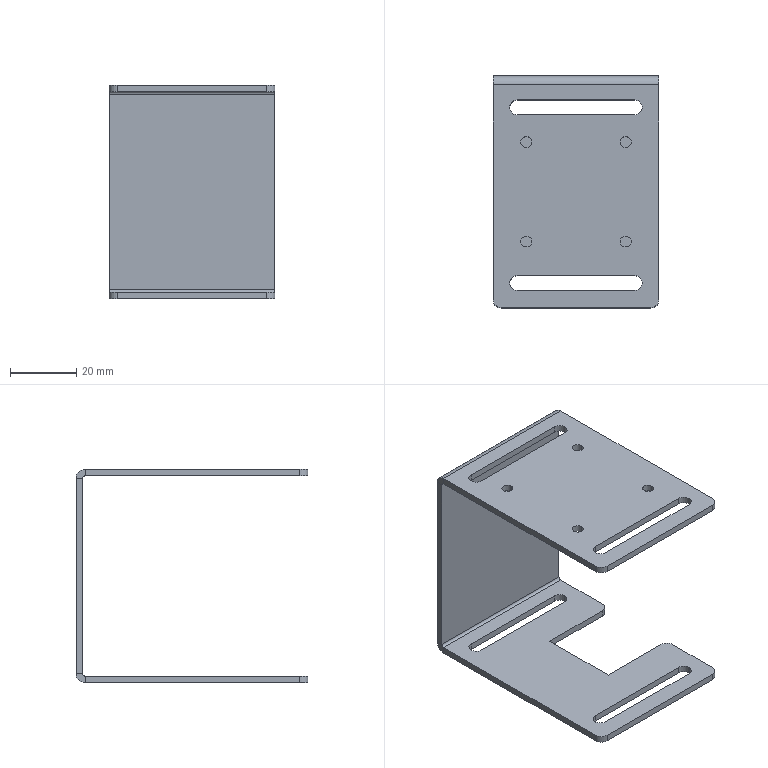Part | SolidWorks | features EdgeFlange 2, HoleWzd 2, Fillet 1, FlatPattern 1, ICE 1, MirrorPattern 1, SMBaseFlange 1, SheetMetal 1 | 1 solid | 60 faces | box 50 x 70 x 64.5 mm | volume 17161 mm3 | cylinder 30 | plane 30 | commonest cylinder face diameters 4.5 x12 3.3 x8 5 x6 1.473 x2 5.473 x2